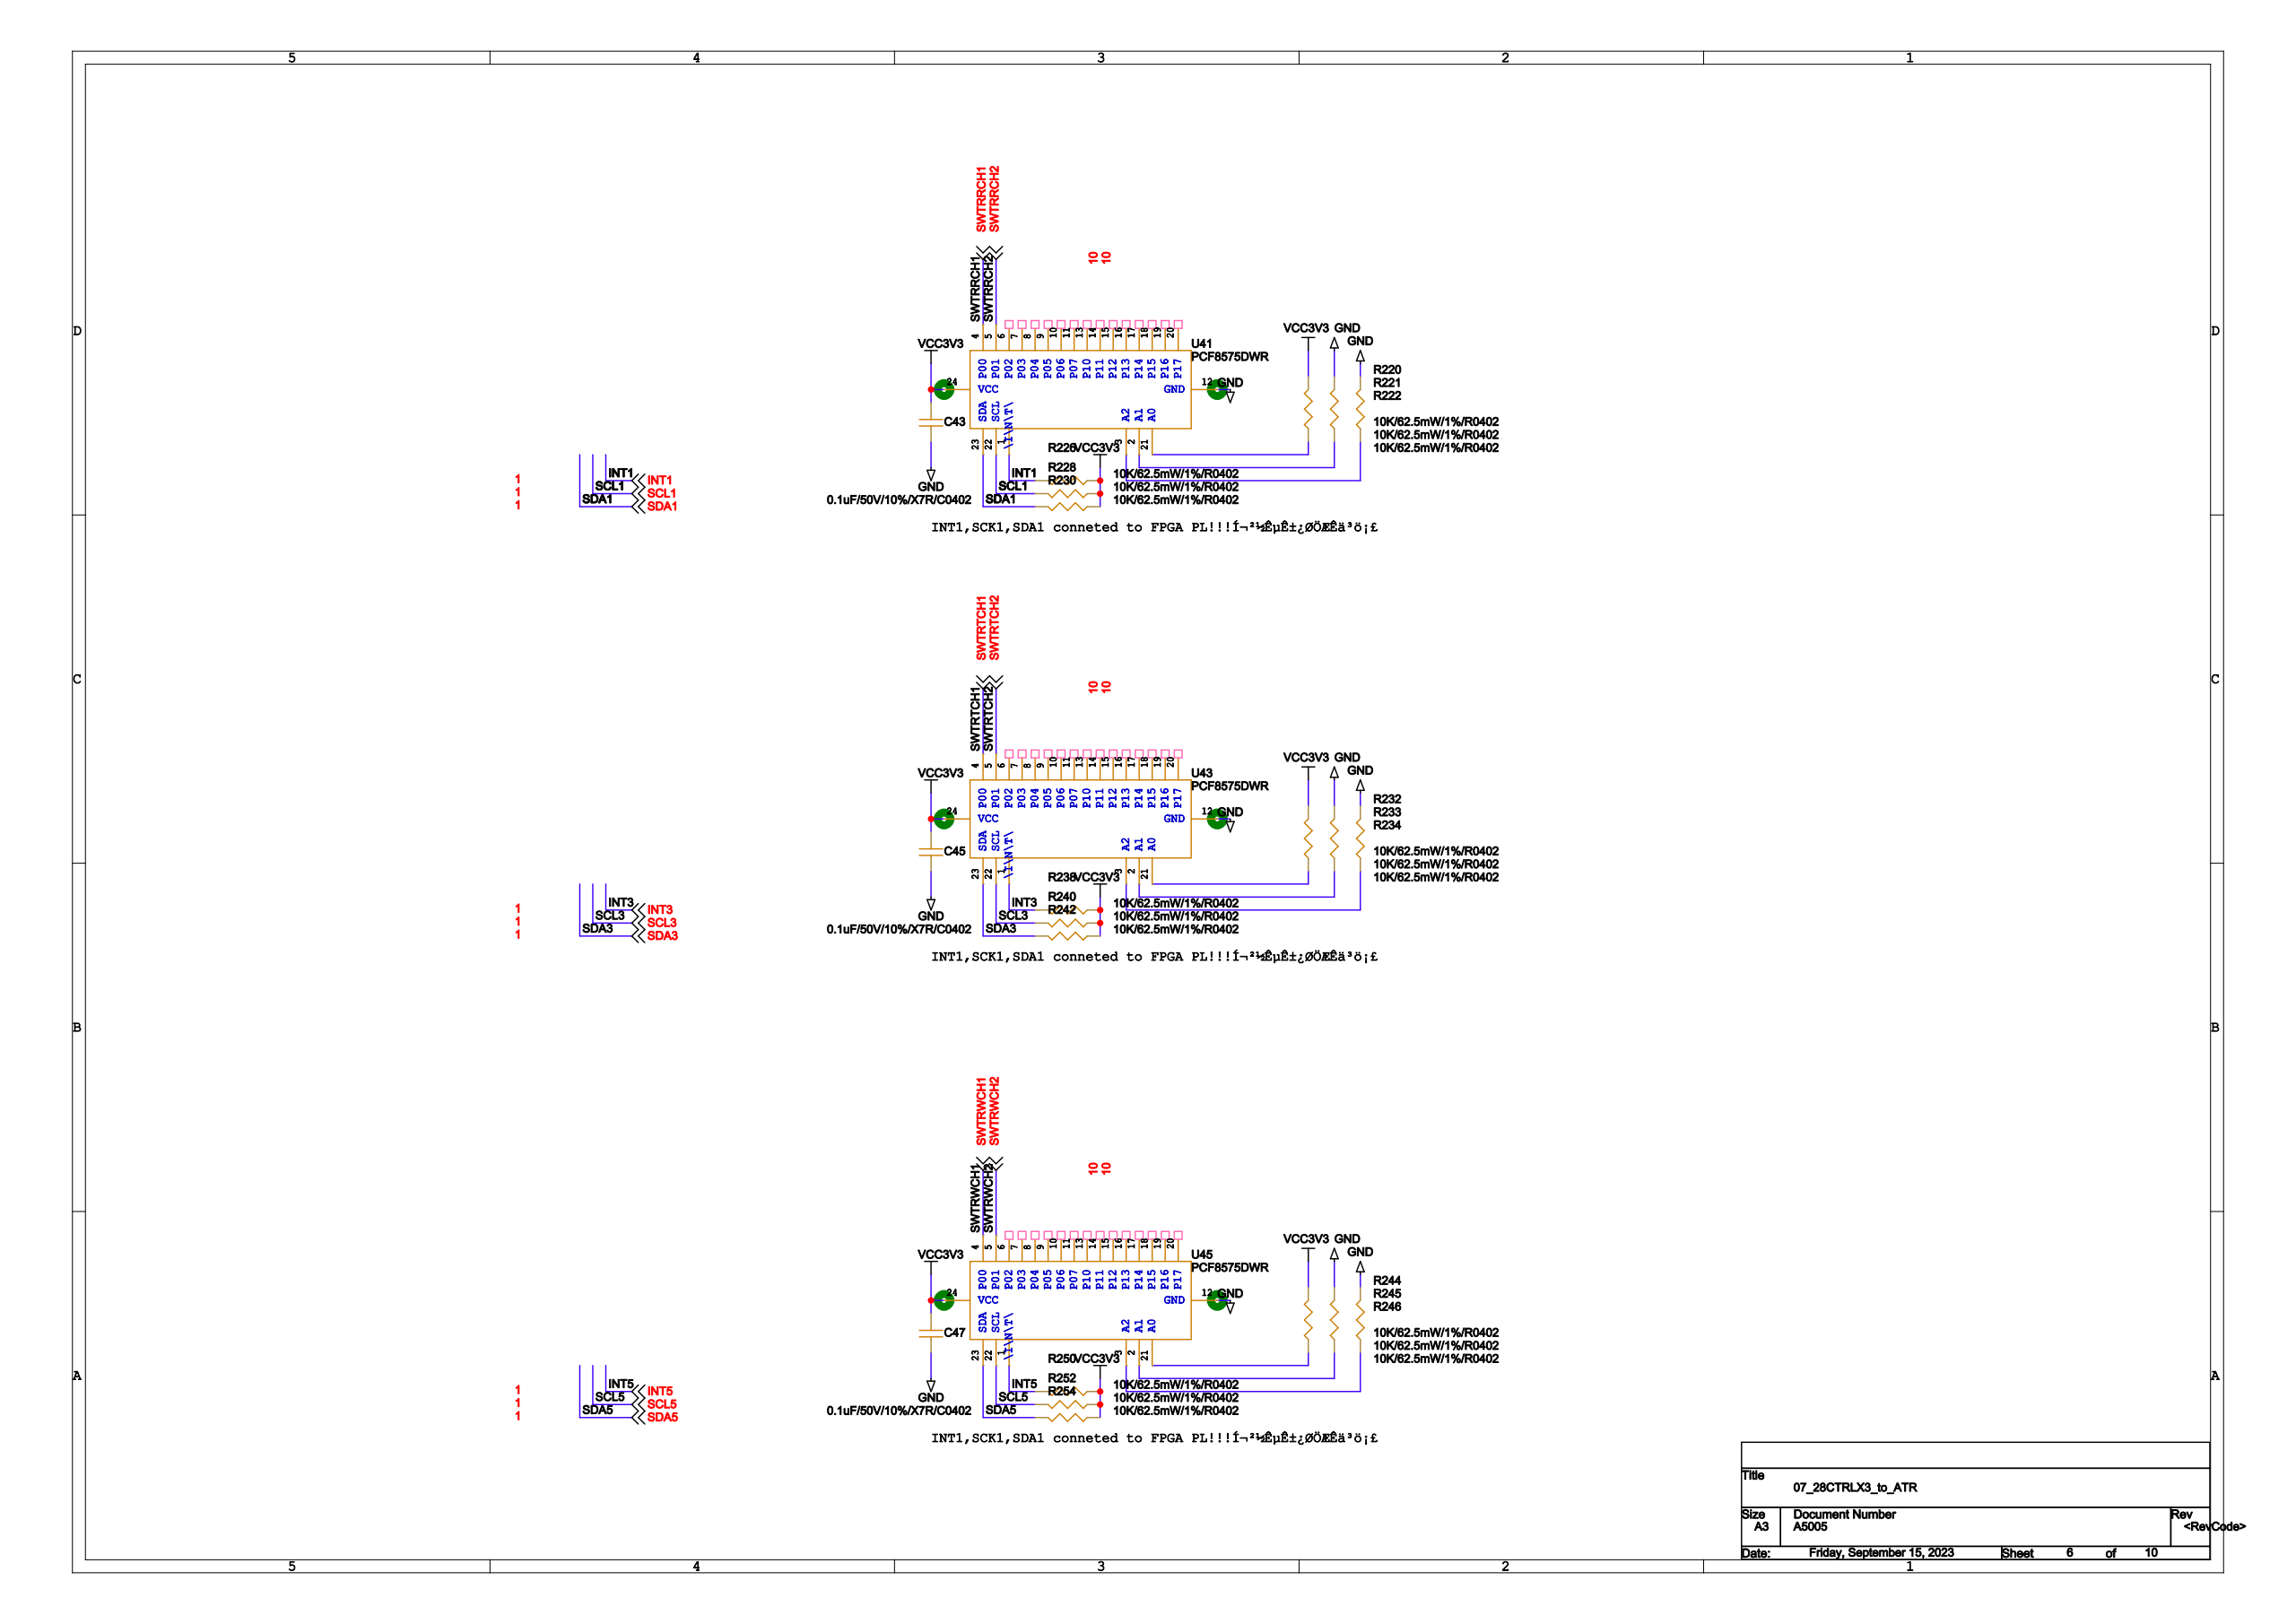Circuit board | Cadence Allegro | 634 parts | 645 nets | one sheet of the schematic
Parts on this sheet (reference | value | footprint):
C43 | 0.1uF/50V/10%/X7R/C0402 | 0402
C45 | 0.1uF/50V/10%/X7R/C0402 | 0402
C47 | 0.1uF/50V/10%/X7R/C0402 | 0402
R220 | 10K/62.5mW/1%/R0402 | 0402
R221 | 10K/62.5mW/1%/R0402 | 0402
R222 | 10K/62.5mW/1%/R0402 | 0402
R226 | 10K/62.5mW/1%/R0402 | 0402
R228 | 10K/62.5mW/1%/R0402 | 0402
R230 | 10K/62.5mW/1%/R0402 | 0402
R232 | 10K/62.5mW/1%/R0402 | 0402
R233 | 10K/62.5mW/1%/R0402 | 0402
R234 | 10K/62.5mW/1%/R0402 | 0402
R238 | 10K/62.5mW/1%/R0402 | 0402
R240 | 10K/62.5mW/1%/R0402 | 0402
R242 | 10K/62.5mW/1%/R0402 | 0402
R244 | 10K/62.5mW/1%/R0402 | 0402
R245 | 10K/62.5mW/1%/R0402 | 0402
R246 | 10K/62.5mW/1%/R0402 | 0402
R250 | 10K/62.5mW/1%/R0402 | 0402
R252 | 10K/62.5mW/1%/R0402 | 0402
R254 | 10K/62.5mW/1%/R0402 | 0402
U41 | PCF8575DWR | SOIC_24
U43 | PCF8575DWR | SOIC_24
U45 | PCF8575DWR | SOIC_24
Nets of these parts (net: part-pin ...):
AGND: C43-1 C45-1 C47-1 R221-1 R222-1 R233-1 R234-1 R245-1 R246-1 U41-12 U43-12 U45-12
3.3V: C43-2 C45-2 C47-2 R220-1 R226-2 R228-2 R230-2 R232-1 R238-2 R240-2 R242-2 R244-1 R250-2 R252-2 R254-2 U41-24 U43-24 U45-24
SDA5: R254-1 U45-23
INT5: R250-1 U45-1
SCL3: R240-1 U43-22
SDA3: R242-1 U43-23
INT3: R238-1 U43-1
INT1: R226-1 U41-1
SDA1: R230-1 U41-23
SCL1: R228-1 U41-22
SCL5: R252-1 U45-22
SWTRRCH1: U41-4
SWTRTCH1: U43-4
SWTRWCH1: U45-4
SWTRRCH2: U41-5
SWTRTCH2: U43-5
SWTRWCH2: U45-5
N23855480: R220-2 U41-21
N23855482: R221-2 U41-2
N23855484: R222-2 U41-3
N23988542: R232-2 U43-21
N23988544: R233-2 U43-2
N23988546: R234-2 U43-3
N23990137: R244-2 U45-21
N23990139: R245-2 U45-2
N23990141: R246-2 U45-3